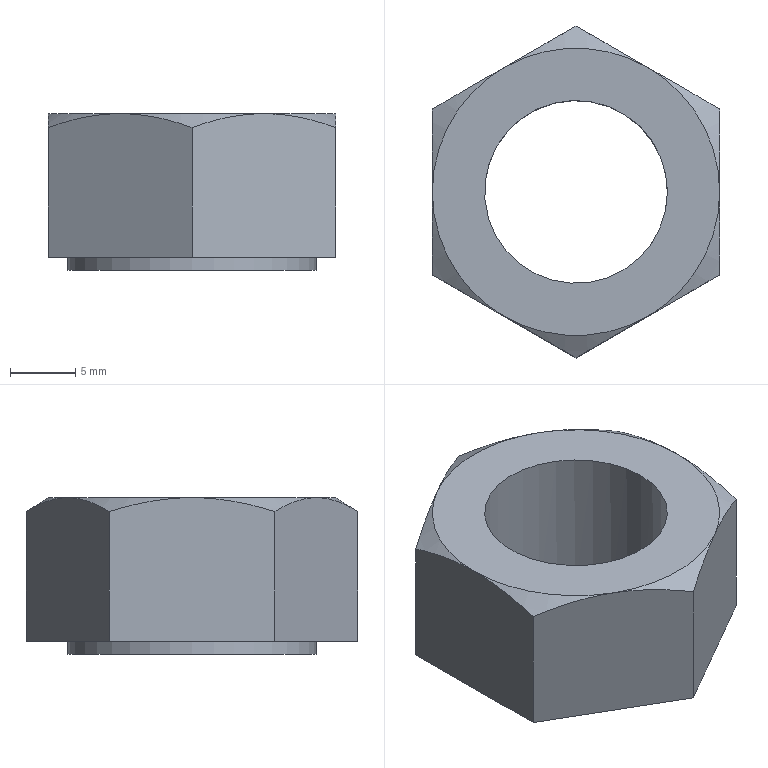Part | NX | features DATUM_CSYS 5, SKETCH 3, EXTRUDE 2, SWP104 1, SYMBOLIC_THREAD 1 | 1 solid | 17 faces | box 22 x 25.403 x 12 mm | volume 3034 mm3 | plane 9 | cone 6 | cylinder 2 | commonest cylinder face diameters 14 x1 19 x1
STEP:
#1=CARTESIAN_POINT('',(-11.,6.351,9.937));
#2=VERTEX_POINT('',#1);
#3=CARTESIAN_POINT('',(-11.,0.,11.));
#4=VERTEX_POINT('',#3);
#5=CARTESIAN_POINT('',(-11.,0.,11.));
#6=CARTESIAN_POINT('',(-11.,2.149,11.));
#7=CARTESIAN_POINT('',(-11.,4.304,10.576));
#8=CARTESIAN_POINT('',(-11.,6.351,9.937));
#9=B_SPLINE_CURVE_WITH_KNOTS('',3,(#5,#6,#7,#8),.UNSPECIFIED.,.F.,.F.,(4,4),(0.0176,0.02404),.UNSPECIFIED.);
#10=EDGE_CURVE('',#2,#4,#9,.F.);
#11=ORIENTED_EDGE('',*,*,#10,.F.);
#12=CARTESIAN_POINT('',(-11.,6.351,0.));
#13=VERTEX_POINT('',#12);
#14=CARTESIAN_POINT('',(-11.,6.351,11.));
#15=DIRECTION('',(0.,0.,-1.));
#16=VECTOR('',#15,1000.);
#17=LINE('',#14,#16);
#18=EDGE_CURVE('',#2,#13,#17,.T.);
#19=ORIENTED_EDGE('',*,*,#18,.T.);
#20=CARTESIAN_POINT('',(-11.,-6.351,0.));
#21=VERTEX_POINT('',#20);
#22=CARTESIAN_POINT('',(-11.,6.351,0.));
#23=DIRECTION('',(0.,-1.,0.));
#24=VECTOR('',#23,1000.);
#25=LINE('',#22,#24);
#26=EDGE_CURVE('',#13,#21,#25,.T.);
#27=ORIENTED_EDGE('',*,*,#26,.T.);
#28=CARTESIAN_POINT('',(-11.,-6.351,9.937));
#29=VERTEX_POINT('',#28);
#30=CARTESIAN_POINT('',(-11.,-6.351,11.));
#31=DIRECTION('',(0.,0.,-1.));
#32=VECTOR('',#31,1000.);
#33=LINE('',#30,#32);
#34=EDGE_CURVE('',#29,#21,#33,.T.);
#35=ORIENTED_EDGE('',*,*,#34,.F.);
#36=CARTESIAN_POINT('',(-11.,-6.351,9.937));
#37=CARTESIAN_POINT('',(-11.,-4.292,10.58));
#38=CARTESIAN_POINT('',(-11.,-2.151,11.));
#39=CARTESIAN_POINT('',(-11.,0.,11.));
#40=B_SPLINE_CURVE_WITH_KNOTS('',3,(#36,#37,#38,#39),.UNSPECIFIED.,.F.,.F.,(4,4),(0.01116,0.0176),.UNSPECIFIED.);
#41=EDGE_CURVE('',#4,#29,#40,.F.);
#42=ORIENTED_EDGE('',*,*,#41,.F.);
#43=EDGE_LOOP('',(#11,#19,#27,#35,#42));
#44=FACE_BOUND('',#43,.T.);
#45=CARTESIAN_POINT('',(-11.,6.351,11.));
#46=DIRECTION('',(1.,0.,0.));
#47=DIRECTION('',(0.,1.,0.));
#48=AXIS2_PLACEMENT_3D('',#45,#46,#47);
#49=PLANE('',#48);
#50=ADVANCED_FACE('',(#44),#49,.F.);
#51=CARTESIAN_POINT('',(-5.5,-9.526,11.));
#52=VERTEX_POINT('',#51);
#53=CARTESIAN_POINT('',(-11.,-6.351,9.937));
#54=CARTESIAN_POINT('',(-9.206,-7.387,10.584));
#55=CARTESIAN_POINT('',(-7.38,-8.441,11.));
#56=CARTESIAN_POINT('',(-5.5,-9.526,11.));
#57=B_SPLINE_CURVE_WITH_KNOTS('',3,(#53,#54,#55,#56),.UNSPECIFIED.,.F.,.F.,(4,4),(0.000000239,0.006439),.UNSPECIFIED.);
#58=EDGE_CURVE('',#29,#52,#57,.T.);
#59=ORIENTED_EDGE('',*,*,#58,.F.);
#60=ORIENTED_EDGE('',*,*,#34,.T.);
#61=CARTESIAN_POINT('',(0.,-12.702,0.));
#62=VERTEX_POINT('',#61);
#63=CARTESIAN_POINT('',(-11.,-6.351,0.));
#64=DIRECTION('',(0.866,-0.5,0.));
#65=VECTOR('',#64,1000.);
#66=LINE('',#63,#65);
#67=EDGE_CURVE('',#21,#62,#66,.T.);
#68=ORIENTED_EDGE('',*,*,#67,.T.);
#69=CARTESIAN_POINT('',(0.,-12.702,9.937));
#70=VERTEX_POINT('',#69);
#71=CARTESIAN_POINT('',(0.,-12.702,11.));
#72=DIRECTION('',(0.,0.,-1.));
#73=VECTOR('',#72,1000.);
#74=LINE('',#71,#73);
#75=EDGE_CURVE('',#70,#62,#74,.T.);
#76=ORIENTED_EDGE('',*,*,#75,.F.);
#77=CARTESIAN_POINT('',(-5.5,-9.526,11.));
#78=CARTESIAN_POINT('',(-3.629,-10.607,11.));
#79=CARTESIAN_POINT('',(-1.788,-11.669,10.582));
#80=CARTESIAN_POINT('',(0.,-12.702,9.937));
#81=B_SPLINE_CURVE_WITH_KNOTS('',3,(#77,#78,#79,#80),.UNSPECIFIED.,.F.,.F.,(4,4),(0.006439,0.01285),.UNSPECIFIED.);
#82=EDGE_CURVE('',#52,#70,#81,.T.);
#83=ORIENTED_EDGE('',*,*,#82,.F.);
#84=EDGE_LOOP('',(#59,#60,#68,#76,#83));
#85=FACE_BOUND('',#84,.T.);
#86=CARTESIAN_POINT('',(-11.,-6.351,11.));
#87=DIRECTION('',(0.5,0.866,0.));
#88=DIRECTION('',(-0.866,0.5,0.));
#89=AXIS2_PLACEMENT_3D('',#86,#87,#88);
#90=PLANE('',#89);
#91=ADVANCED_FACE('',(#85),#90,.F.);
#92=CARTESIAN_POINT('',(5.5,-9.526,11.));
#93=VERTEX_POINT('',#92);
#94=CARTESIAN_POINT('',(0.,-12.702,9.937));
#95=CARTESIAN_POINT('',(1.794,-11.666,10.584));
#96=CARTESIAN_POINT('',(3.62,-10.612,11.));
#97=CARTESIAN_POINT('',(5.5,-9.526,11.));
#98=B_SPLINE_CURVE_WITH_KNOTS('',3,(#94,#95,#96,#97),.UNSPECIFIED.,.F.,.F.,(4,4),(0.000000239,0.006439),.UNSPECIFIED.);
#99=EDGE_CURVE('',#70,#93,#98,.T.);
#100=ORIENTED_EDGE('',*,*,#99,.F.);
#101=ORIENTED_EDGE('',*,*,#75,.T.);
#102=CARTESIAN_POINT('',(11.,-6.351,0.));
#103=VERTEX_POINT('',#102);
#104=CARTESIAN_POINT('',(0.,-12.702,0.));
#105=DIRECTION('',(0.866,0.5,0.));
#106=VECTOR('',#105,1000.);
#107=LINE('',#104,#106);
#108=EDGE_CURVE('',#62,#103,#107,.T.);
#109=ORIENTED_EDGE('',*,*,#108,.T.);
#110=CARTESIAN_POINT('',(11.,-6.351,9.937));
#111=VERTEX_POINT('',#110);
#112=CARTESIAN_POINT('',(11.,-6.351,11.));
#113=DIRECTION('',(0.,0.,-1.));
#114=VECTOR('',#113,1000.);
#115=LINE('',#112,#114);
#116=EDGE_CURVE('',#111,#103,#115,.T.);
#117=ORIENTED_EDGE('',*,*,#116,.F.);
#118=CARTESIAN_POINT('',(5.5,-9.526,11.));
#119=CARTESIAN_POINT('',(7.371,-8.446,11.));
#120=CARTESIAN_POINT('',(9.212,-7.383,10.582));
#121=CARTESIAN_POINT('',(11.,-6.351,9.937));
#122=B_SPLINE_CURVE_WITH_KNOTS('',3,(#118,#119,#120,#121),.UNSPECIFIED.,.F.,.F.,(4,4),(0.006439,0.01285),.UNSPECIFIED.);
#123=EDGE_CURVE('',#93,#111,#122,.T.);
#124=ORIENTED_EDGE('',*,*,#123,.F.);
#125=EDGE_LOOP('',(#100,#101,#109,#117,#124));
#126=FACE_BOUND('',#125,.T.);
#127=CARTESIAN_POINT('',(0.,-12.702,11.));
#128=DIRECTION('',(-0.5,0.866,0.));
#129=DIRECTION('',(-0.866,-0.5,0.));
#130=AXIS2_PLACEMENT_3D('',#127,#128,#129);
#131=PLANE('',#130);
#132=ADVANCED_FACE('',(#126),#131,.F.);
#133=CARTESIAN_POINT('',(11.,0.,11.));
#134=VERTEX_POINT('',#133);
#135=CARTESIAN_POINT('',(11.,-6.351,9.937));
#136=CARTESIAN_POINT('',(11.,-4.292,10.58));
#137=CARTESIAN_POINT('',(11.,-2.151,11.));
#138=CARTESIAN_POINT('',(11.,0.,11.));
#139=B_SPLINE_CURVE_WITH_KNOTS('',3,(#135,#136,#137,#138),.UNSPECIFIED.,.F.,.F.,(4,4),(0.01116,0.0176),.UNSPECIFIED.);
#140=EDGE_CURVE('',#111,#134,#139,.T.);
#141=ORIENTED_EDGE('',*,*,#140,.F.);
#142=ORIENTED_EDGE('',*,*,#116,.T.);
#143=CARTESIAN_POINT('',(11.,6.351,0.));
#144=VERTEX_POINT('',#143);
#145=CARTESIAN_POINT('',(11.,-6.351,0.));
#146=DIRECTION('',(0.,1.,0.));
#147=VECTOR('',#146,1000.);
#148=LINE('',#145,#147);
#149=EDGE_CURVE('',#103,#144,#148,.T.);
#150=ORIENTED_EDGE('',*,*,#149,.T.);
#151=CARTESIAN_POINT('',(11.,6.351,9.937));
#152=VERTEX_POINT('',#151);
#153=CARTESIAN_POINT('',(11.,6.351,11.));
#154=DIRECTION('',(0.,0.,-1.));
#155=VECTOR('',#154,1000.);
#156=LINE('',#153,#155);
#157=EDGE_CURVE('',#152,#144,#156,.T.);
#158=ORIENTED_EDGE('',*,*,#157,.F.);
#159=CARTESIAN_POINT('',(11.,0.,11.));
#160=CARTESIAN_POINT('',(11.,2.149,11.));
#161=CARTESIAN_POINT('',(11.,4.304,10.576));
#162=CARTESIAN_POINT('',(11.,6.351,9.937));
#163=B_SPLINE_CURVE_WITH_KNOTS('',3,(#159,#160,#161,#162),.UNSPECIFIED.,.F.,.F.,(4,4),(0.0176,0.02404),.UNSPECIFIED.);
#164=EDGE_CURVE('',#134,#152,#163,.T.);
#165=ORIENTED_EDGE('',*,*,#164,.F.);
#166=EDGE_LOOP('',(#141,#142,#150,#158,#165));
#167=FACE_BOUND('',#166,.T.);
#168=CARTESIAN_POINT('',(11.,-6.351,11.));
#169=DIRECTION('',(-1.,0.,0.));
#170=DIRECTION('',(0.,-1.,0.));
#171=AXIS2_PLACEMENT_3D('',#168,#169,#170);
#172=PLANE('',#171);
#173=ADVANCED_FACE('',(#167),#172,.F.);
#174=CARTESIAN_POINT('',(5.5,9.526,11.));
#175=VERTEX_POINT('',#174);
#176=CARTESIAN_POINT('',(11.,6.351,9.937));
#177=CARTESIAN_POINT('',(9.206,7.387,10.584));
#178=CARTESIAN_POINT('',(7.38,8.441,11.));
#179=CARTESIAN_POINT('',(5.5,9.526,11.));
#180=B_SPLINE_CURVE_WITH_KNOTS('',3,(#176,#177,#178,#179),.UNSPECIFIED.,.F.,.F.,(4,4),(0.000000239,0.006439),.UNSPECIFIED.);
#181=EDGE_CURVE('',#152,#175,#180,.T.);
#182=ORIENTED_EDGE('',*,*,#181,.F.);
#183=ORIENTED_EDGE('',*,*,#157,.T.);
#184=CARTESIAN_POINT('',(0.,12.702,0.));
#185=VERTEX_POINT('',#184);
#186=CARTESIAN_POINT('',(11.,6.351,0.));
#187=DIRECTION('',(-0.866,0.5,0.));
#188=VECTOR('',#187,1000.);
#189=LINE('',#186,#188);
#190=EDGE_CURVE('',#144,#185,#189,.T.);
#191=ORIENTED_EDGE('',*,*,#190,.T.);
#192=CARTESIAN_POINT('',(0.,12.702,9.937));
#193=VERTEX_POINT('',#192);
#194=CARTESIAN_POINT('',(0.,12.702,11.));
#195=DIRECTION('',(0.,0.,-1.));
#196=VECTOR('',#195,1000.);
#197=LINE('',#194,#196);
#198=EDGE_CURVE('',#193,#185,#197,.T.);
#199=ORIENTED_EDGE('',*,*,#198,.F.);
#200=CARTESIAN_POINT('',(5.5,9.526,11.));
#201=CARTESIAN_POINT('',(3.629,10.607,11.));
#202=CARTESIAN_POINT('',(1.788,11.669,10.582));
#203=CARTESIAN_POINT('',(0.,12.702,9.937));
#204=B_SPLINE_CURVE_WITH_KNOTS('',3,(#200,#201,#202,#203),.UNSPECIFIED.,.F.,.F.,(4,4),(0.006439,0.01285),.UNSPECIFIED.);
#205=EDGE_CURVE('',#175,#193,#204,.T.);
#206=ORIENTED_EDGE('',*,*,#205,.F.);
#207=EDGE_LOOP('',(#182,#183,#191,#199,#206));
#208=FACE_BOUND('',#207,.T.);
#209=CARTESIAN_POINT('',(11.,6.351,11.));
#210=DIRECTION('',(-0.5,-0.866,0.));
#211=DIRECTION('',(0.866,-0.5,0.));
#212=AXIS2_PLACEMENT_3D('',#209,#210,#211);
#213=PLANE('',#212);
#214=ADVANCED_FACE('',(#208),#213,.F.);
#215=CARTESIAN_POINT('',(-5.5,9.526,11.));
#216=VERTEX_POINT('',#215);
#217=CARTESIAN_POINT('',(0.,12.702,9.937));
#218=CARTESIAN_POINT('',(-1.794,11.666,10.584));
#219=CARTESIAN_POINT('',(-3.62,10.612,11.));
#220=CARTESIAN_POINT('',(-5.5,9.526,11.));
#221=B_SPLINE_CURVE_WITH_KNOTS('',3,(#217,#218,#219,#220),.UNSPECIFIED.,.F.,.F.,(4,4),(0.000000239,0.006439),.UNSPECIFIED.);
#222=EDGE_CURVE('',#193,#216,#221,.T.);
#223=ORIENTED_EDGE('',*,*,#222,.F.);
#224=ORIENTED_EDGE('',*,*,#198,.T.);
#225=CARTESIAN_POINT('',(0.,12.702,0.));
#226=DIRECTION('',(-0.866,-0.5,0.));
#227=VECTOR('',#226,1000.);
#228=LINE('',#225,#227);
#229=EDGE_CURVE('',#185,#13,#228,.T.);
#230=ORIENTED_EDGE('',*,*,#229,.T.);
#231=ORIENTED_EDGE('',*,*,#18,.F.);
#232=CARTESIAN_POINT('',(-5.5,9.526,11.));
#233=CARTESIAN_POINT('',(-7.371,8.446,11.));
#234=CARTESIAN_POINT('',(-9.212,7.383,10.582));
#235=CARTESIAN_POINT('',(-11.,6.351,9.937));
#236=B_SPLINE_CURVE_WITH_KNOTS('',3,(#232,#233,#234,#235),.UNSPECIFIED.,.F.,.F.,(4,4),(0.006439,0.01285),.UNSPECIFIED.);
#237=EDGE_CURVE('',#216,#2,#236,.T.);
#238=ORIENTED_EDGE('',*,*,#237,.F.);
#239=EDGE_LOOP('',(#223,#224,#230,#231,#238));
#240=FACE_BOUND('',#239,.T.);
#241=CARTESIAN_POINT('',(0.,12.702,11.));
#242=DIRECTION('',(0.5,-0.866,0.));
#243=DIRECTION('',(0.866,0.5,0.));
#244=AXIS2_PLACEMENT_3D('',#241,#242,#243);
#245=PLANE('',#244);
#246=ADVANCED_FACE('',(#240),#245,.F.);
#247=CARTESIAN_POINT('',(7.,0.,11.));
#248=VERTEX_POINT('',#247);
#249=CARTESIAN_POINT('',(0.,0.,11.));
#250=DIRECTION('',(0.,0.,1.));
#251=DIRECTION('',(1.,0.,0.));
#252=AXIS2_PLACEMENT_3D('',#249,#250,#251);
#253=CIRCLE('',#252,7.);
#254=EDGE_CURVE('',#248,#248,#253,.T.);
#255=ORIENTED_EDGE('',*,*,#254,.F.);
#256=EDGE_LOOP('',(#255));
#257=FACE_BOUND('',#256,.T.);
#258=CARTESIAN_POINT('',(0.,0.,11.));
#259=DIRECTION('',(0.,0.,1.));
#260=DIRECTION('',(1.,0.,0.));
#261=AXIS2_PLACEMENT_3D('',#258,#259,#260);
#262=CIRCLE('',#261,11.);
#263=EDGE_CURVE('',#93,#134,#262,.T.);
#264=ORIENTED_EDGE('',*,*,#263,.T.);
#265=CARTESIAN_POINT('',(0.,0.,11.));
#266=DIRECTION('',(0.,0.,1.));
#267=DIRECTION('',(1.,0.,0.));
#268=AXIS2_PLACEMENT_3D('',#265,#266,#267);
#269=CIRCLE('',#268,11.);
#270=EDGE_CURVE('',#134,#175,#269,.T.);
#271=ORIENTED_EDGE('',*,*,#270,.T.);
#272=CARTESIAN_POINT('',(0.,0.,11.));
#273=DIRECTION('',(0.,0.,1.));
#274=DIRECTION('',(1.,0.,0.));
#275=AXIS2_PLACEMENT_3D('',#272,#273,#274);
#276=CIRCLE('',#275,11.);
#277=EDGE_CURVE('',#175,#216,#276,.T.);
#278=ORIENTED_EDGE('',*,*,#277,.T.);
#279=CARTESIAN_POINT('',(0.,0.,11.));
#280=DIRECTION('',(0.,0.,1.));
#281=DIRECTION('',(1.,0.,0.));
#282=AXIS2_PLACEMENT_3D('',#279,#280,#281);
#283=CIRCLE('',#282,11.);
#284=EDGE_CURVE('',#216,#4,#283,.T.);
#285=ORIENTED_EDGE('',*,*,#284,.T.);
#286=CARTESIAN_POINT('',(0.,0.,11.));
#287=DIRECTION('',(0.,0.,1.));
#288=DIRECTION('',(1.,0.,0.));
#289=AXIS2_PLACEMENT_3D('',#286,#287,#288);
#290=CIRCLE('',#289,11.);
#291=EDGE_CURVE('',#4,#52,#290,.T.);
#292=ORIENTED_EDGE('',*,*,#291,.T.);
#293=CARTESIAN_POINT('',(0.,0.,11.));
#294=DIRECTION('',(0.,0.,1.));
#295=DIRECTION('',(1.,0.,0.));
#296=AXIS2_PLACEMENT_3D('',#293,#294,#295);
#297=CIRCLE('',#296,11.);
#298=EDGE_CURVE('',#52,#93,#297,.T.);
#299=ORIENTED_EDGE('',*,*,#298,.T.);
#300=EDGE_LOOP('',(#264,#271,#278,#285,#292,#299));
#301=FACE_BOUND('',#300,.T.);
#302=CARTESIAN_POINT('',(0.,0.,11.));
#303=DIRECTION('',(0.,0.,1.));
#304=DIRECTION('',(1.,0.,0.));
#305=AXIS2_PLACEMENT_3D('',#302,#303,#304);
#306=PLANE('',#305);
#307=ADVANCED_FACE('',(#257,#301),#306,.T.);
#308=ORIENTED_EDGE('',*,*,#26,.F.);
#309=ORIENTED_EDGE('',*,*,#229,.F.);
#310=ORIENTED_EDGE('',*,*,#190,.F.);
#311=ORIENTED_EDGE('',*,*,#149,.F.);
#312=ORIENTED_EDGE('',*,*,#108,.F.);
#313=ORIENTED_EDGE('',*,*,#67,.F.);
#314=EDGE_LOOP('',(#308,#309,#310,#311,#312,#313));
#315=FACE_BOUND('',#314,.T.);
#316=CARTESIAN_POINT('',(-8.227,4.75,0.));
#317=VERTEX_POINT('',#316);
#318=CARTESIAN_POINT('',(0.,0.,0.));
#319=DIRECTION('',(0.,0.,-1.));
#320=DIRECTION('',(-0.866,0.5,0.));
#321=AXIS2_PLACEMENT_3D('',#318,#319,#320);
#322=CIRCLE('',#321,9.5);
#323=EDGE_CURVE('',#317,#317,#322,.T.);
#324=ORIENTED_EDGE('',*,*,#323,.F.);
#325=EDGE_LOOP('',(#324));
#326=FACE_BOUND('',#325,.T.);
#327=CARTESIAN_POINT('',(0.,0.,0.));
#328=DIRECTION('',(0.,0.,1.));
#329=DIRECTION('',(1.,0.,0.));
#330=AXIS2_PLACEMENT_3D('',#327,#328,#329);
#331=PLANE('',#330);
#332=ADVANCED_FACE('',(#315,#326),#331,.F.);
#333=ORIENTED_EDGE('',*,*,#254,.T.);
#334=EDGE_LOOP('',(#333));
#335=FACE_BOUND('',#334,.T.);
#336=CARTESIAN_POINT('',(-6.062,3.5,-1.));
#337=VERTEX_POINT('',#336);
#338=CARTESIAN_POINT('',(0.,0.,-1.));
#339=DIRECTION('',(0.,0.,-1.));
#340=DIRECTION('',(-0.866,0.5,0.));
#341=AXIS2_PLACEMENT_3D('',#338,#339,#340);
#342=CIRCLE('',#341,7.);
#343=EDGE_CURVE('',#337,#337,#342,.T.);
#344=ORIENTED_EDGE('',*,*,#343,.T.);
#345=EDGE_LOOP('',(#344));
#346=FACE_BOUND('',#345,.T.);
#347=CARTESIAN_POINT('',(0.,0.,11.));
#348=DIRECTION('',(0.,0.,-1.));
#349=DIRECTION('',(-1.,0.,0.));
#350=AXIS2_PLACEMENT_3D('',#347,#348,#349);
#351=CYLINDRICAL_SURFACE('',#350,7.);
#352=ADVANCED_FACE('',(#335,#346),#351,.F.);
#353=CARTESIAN_POINT('',(-8.227,4.75,-1.));
#354=VERTEX_POINT('',#353);
#355=CARTESIAN_POINT('',(0.,0.,-1.));
#356=DIRECTION('',(0.,0.,-1.));
#357=DIRECTION('',(-0.866,0.5,0.));
#358=AXIS2_PLACEMENT_3D('',#355,#356,#357);
#359=CIRCLE('',#358,9.5);
#360=EDGE_CURVE('',#354,#354,#359,.T.);
#361=ORIENTED_EDGE('',*,*,#360,.F.);
#362=EDGE_LOOP('',(#361));
#363=FACE_BOUND('',#362,.T.);
#364=ORIENTED_EDGE('',*,*,#323,.T.);
#365=EDGE_LOOP('',(#364));
#366=FACE_BOUND('',#365,.T.);
#367=CARTESIAN_POINT('',(0.,0.,-1.));
#368=DIRECTION('',(0.,0.,1.));
#369=DIRECTION('',(1.,0.,0.));
#370=AXIS2_PLACEMENT_3D('',#367,#368,#369);
#371=CYLINDRICAL_SURFACE('',#370,9.5);
#372=ADVANCED_FACE('',(#363,#366),#371,.T.);
#373=ORIENTED_EDGE('',*,*,#360,.T.);
#374=EDGE_LOOP('',(#373));
#375=FACE_BOUND('',#374,.T.);
#376=ORIENTED_EDGE('',*,*,#343,.F.);
#377=EDGE_LOOP('',(#376));
#378=FACE_BOUND('',#377,.T.);
#379=CARTESIAN_POINT('',(0.,0.,-1.));
#380=DIRECTION('',(0.,0.,-1.));
#381=DIRECTION('',(-1.,0.,0.));
#382=AXIS2_PLACEMENT_3D('',#379,#380,#381);
#383=PLANE('',#382);
#384=ADVANCED_FACE('',(#375,#378),#383,.T.);
#385=ORIENTED_EDGE('',*,*,#140,.T.);
#386=ORIENTED_EDGE('',*,*,#263,.F.);
#387=ORIENTED_EDGE('',*,*,#123,.T.);
#388=EDGE_LOOP('',(#385,#386,#387));
#389=FACE_BOUND('',#388,.T.);
#390=CARTESIAN_POINT('',(0.,0.,9.675));
#391=DIRECTION('',(0.,0.,-1.));
#392=DIRECTION('',(-1.,0.,0.));
#393=AXIS2_PLACEMENT_3D('',#390,#391,#392);
#394=CONICAL_SURFACE('',#393,13.12,1.012);
#395=ADVANCED_FACE('',(#389),#394,.T.);
#396=ORIENTED_EDGE('',*,*,#99,.T.);
#397=ORIENTED_EDGE('',*,*,#298,.F.);
#398=ORIENTED_EDGE('',*,*,#82,.T.);
#399=EDGE_LOOP('',(#396,#397,#398));
#400=FACE_BOUND('',#399,.T.);
#401=CARTESIAN_POINT('',(0.,0.,9.675));
#402=DIRECTION('',(0.,0.,-1.));
#403=DIRECTION('',(-1.,0.,0.));
#404=AXIS2_PLACEMENT_3D('',#401,#402,#403);
#405=CONICAL_SURFACE('',#404,13.12,1.012);
#406=ADVANCED_FACE('',(#400),#405,.T.);
#407=ORIENTED_EDGE('',*,*,#58,.T.);
#408=ORIENTED_EDGE('',*,*,#291,.F.);
#409=ORIENTED_EDGE('',*,*,#41,.T.);
#410=EDGE_LOOP('',(#407,#408,#409));
#411=FACE_BOUND('',#410,.T.);
#412=CARTESIAN_POINT('',(0.,0.,9.675));
#413=DIRECTION('',(0.,0.,-1.));
#414=DIRECTION('',(-1.,0.,0.));
#415=AXIS2_PLACEMENT_3D('',#412,#413,#414);
#416=CONICAL_SURFACE('',#415,13.12,1.012);
#417=ADVANCED_FACE('',(#411),#416,.T.);
#418=ORIENTED_EDGE('',*,*,#10,.T.);
#419=ORIENTED_EDGE('',*,*,#284,.F.);
#420=ORIENTED_EDGE('',*,*,#237,.T.);
#421=EDGE_LOOP('',(#418,#419,#420));
#422=FACE_BOUND('',#421,.T.);
#423=CARTESIAN_POINT('',(0.,0.,9.675));
#424=DIRECTION('',(0.,0.,-1.));
#425=DIRECTION('',(-1.,0.,0.));
#426=AXIS2_PLACEMENT_3D('',#423,#424,#425);
#427=CONICAL_SURFACE('',#426,13.12,1.012);
#428=ADVANCED_FACE('',(#422),#427,.T.);
#429=ORIENTED_EDGE('',*,*,#222,.T.);
#430=ORIENTED_EDGE('',*,*,#277,.F.);
#431=ORIENTED_EDGE('',*,*,#205,.T.);
#432=EDGE_LOOP('',(#429,#430,#431));
#433=FACE_BOUND('',#432,.T.);
#434=CARTESIAN_POINT('',(0.,0.,9.675));
#435=DIRECTION('',(0.,0.,-1.));
#436=DIRECTION('',(-1.,0.,0.));
#437=AXIS2_PLACEMENT_3D('',#434,#435,#436);
#438=CONICAL_SURFACE('',#437,13.12,1.012);
#439=ADVANCED_FACE('',(#433),#438,.T.);
#440=ORIENTED_EDGE('',*,*,#181,.T.);
#441=ORIENTED_EDGE('',*,*,#270,.F.);
#442=ORIENTED_EDGE('',*,*,#164,.T.);
#443=EDGE_LOOP('',(#440,#441,#442));
#444=FACE_BOUND('',#443,.T.);
#445=CARTESIAN_POINT('',(0.,0.,9.675));
#446=DIRECTION('',(0.,0.,-1.));
#447=DIRECTION('',(-1.,0.,0.));
#448=AXIS2_PLACEMENT_3D('',#445,#446,#447);
#449=CONICAL_SURFACE('',#448,13.12,1.012);
#450=ADVANCED_FACE('',(#444),#449,.T.);
#451=CLOSED_SHELL('',(#50,#91,#132,#173,#214,#246,#307,#332,#352,#372,#384,#395,#406,#417,#428,#439,#450));
#452=MANIFOLD_SOLID_BREP('',#451);
#453=(LENGTH_UNIT()NAMED_UNIT(*)SI_UNIT(.MILLI.,.METRE.));
#454=UNCERTAINTY_MEASURE_WITH_UNIT(LENGTH_MEASURE(0.0508),#453,'','');
#455=(NAMED_UNIT(*)PLANE_ANGLE_UNIT()SI_UNIT($,.RADIAN.));
#456=(NAMED_UNIT(*)SI_UNIT($,.STERADIAN.)SOLID_ANGLE_UNIT());
#457=(GEOMETRIC_REPRESENTATION_CONTEXT(3)GLOBAL_UNCERTAINTY_ASSIGNED_CONTEXT((#454))GLOBAL_UNIT_ASSIGNED_CONTEXT((#453,#455,#456))REPRESENTATION_CONTEXT('',''));
#458=ADVANCED_BREP_SHAPE_REPRESENTATION('',(#452),#457);